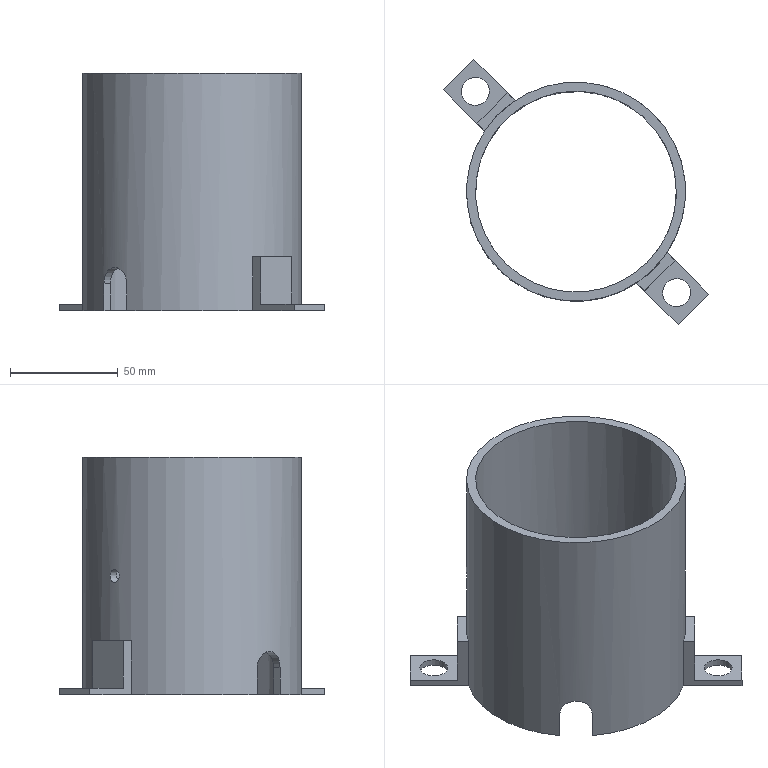Part | NX | features solid 2 | 1 solid | 26 faces | box 123.037 x 123.037 x 110 mm | volume 145297 mm3 | plane 19 | cylinder 7 | commonest cylinder face diameters 13 x2 15 x2 6 x1 93.2 x1 101.6 x1
STEP:
#1=CARTESIAN_POINT('',(-1217.073,-302.927,-100.));
#2=VERTEX_POINT('',#1);
#3=CARTESIAN_POINT('',(-1221.669,-298.331,-100.));
#4=DIRECTION('',(0.,0.,1.));
#5=DIRECTION('',(0.7071,-0.7071,0.));
#6=AXIS2_PLACEMENT_3D('',#3,#4,#5);
#7=CIRCLE('',#6,6.5);
#8=EDGE_CURVE('',#2,#2,#7,.T.);
#9=ORIENTED_EDGE('',*,*,#8,.T.);
#10=EDGE_LOOP('',(#9));
#11=FACE_BOUND('',#10,.T.);
#12=CARTESIAN_POINT('',(-1144.776,-304.169,-100.));
#13=VERTEX_POINT('',#12);
#14=CARTESIAN_POINT('',(-1203.147,-302.711,-100.));
#15=VERTEX_POINT('',#14);
#16=CARTESIAN_POINT('',(-1175.,-345.,-100.));
#17=DIRECTION('',(0.,0.,1.));
#18=DIRECTION('',(0.7071,-0.7071,0.));
#19=AXIS2_PLACEMENT_3D('',#16,#17,#18);
#20=CIRCLE('',#19,50.8);
#21=EDGE_CURVE('',#13,#15,#20,.T.);
#22=ORIENTED_EDGE('',*,*,#21,.F.);
#23=CARTESIAN_POINT('',(-1147.782,-307.175,-100.));
#24=VERTEX_POINT('',#23);
#25=CARTESIAN_POINT('',(-1180.303,-339.697,-100.));
#26=DIRECTION('',(-0.7071,-0.7071,0.));
#27=VECTOR('',#26,1000.);
#28=LINE('',#25,#27);
#29=EDGE_CURVE('',#13,#24,#28,.T.);
#30=ORIENTED_EDGE('',*,*,#29,.T.);
#31=CARTESIAN_POINT('',(-1212.825,-372.218,-100.));
#32=VERTEX_POINT('',#31);
#33=CARTESIAN_POINT('',(-1175.,-345.,-100.));
#34=DIRECTION('',(0.,0.,1.));
#35=DIRECTION('',(0.7071,-0.7071,0.));
#36=AXIS2_PLACEMENT_3D('',#33,#34,#35);
#37=CIRCLE('',#36,46.6);
#38=EDGE_CURVE('',#24,#32,#37,.T.);
#39=ORIENTED_EDGE('',*,*,#38,.T.);
#40=CARTESIAN_POINT('',(-1215.831,-375.224,-100.));
#41=VERTEX_POINT('',#40);
#42=CARTESIAN_POINT('',(-1180.303,-339.697,-100.));
#43=DIRECTION('',(-0.7071,-0.7071,0.));
#44=VECTOR('',#43,1000.);
#45=LINE('',#42,#44);
#46=EDGE_CURVE('',#32,#41,#45,.T.);
#47=ORIENTED_EDGE('',*,*,#46,.T.);
#48=CARTESIAN_POINT('',(-1217.289,-316.853,-100.));
#49=VERTEX_POINT('',#48);
#50=CARTESIAN_POINT('',(-1175.,-345.,-100.));
#51=DIRECTION('',(0.,0.,1.));
#52=DIRECTION('',(0.7071,-0.7071,0.));
#53=AXIS2_PLACEMENT_3D('',#50,#51,#52);
#54=CIRCLE('',#53,50.8);
#55=EDGE_CURVE('',#49,#41,#54,.T.);
#56=ORIENTED_EDGE('',*,*,#55,.F.);
#57=CARTESIAN_POINT('',(-1236.518,-297.624,-100.));
#58=VERTEX_POINT('',#57);
#59=CARTESIAN_POINT('',(-1226.619,-307.523,-100.));
#60=DIRECTION('',(0.7071,-0.7071,0.));
#61=VECTOR('',#60,1000.);
#62=LINE('',#59,#61);
#63=EDGE_CURVE('',#58,#49,#62,.T.);
#64=ORIENTED_EDGE('',*,*,#63,.F.);
#65=CARTESIAN_POINT('',(-1222.376,-283.482,-100.));
#66=VERTEX_POINT('',#65);
#67=CARTESIAN_POINT('',(-1236.518,-297.624,-100.));
#68=DIRECTION('',(0.7071,0.7071,0.));
#69=VECTOR('',#68,1000.);
#70=LINE('',#67,#69);
#71=EDGE_CURVE('',#58,#66,#70,.T.);
#72=ORIENTED_EDGE('',*,*,#71,.T.);
#73=CARTESIAN_POINT('',(-1206.113,-299.745,-100.));
#74=DIRECTION('',(-0.7071,0.7071,0.));
#75=VECTOR('',#74,1000.);
#76=LINE('',#73,#75);
#77=EDGE_CURVE('',#15,#66,#76,.T.);
#78=ORIENTED_EDGE('',*,*,#77,.F.);
#79=EDGE_LOOP('',(#22,#30,#39,#47,#56,#64,#72,#78));
#80=FACE_BOUND('',#79,.T.);
#81=CARTESIAN_POINT('',(-1175.,-345.,-100.));
#82=DIRECTION('',(0.,0.,1.));
#83=DIRECTION('',(0.7071,-0.7071,0.));
#84=AXIS2_PLACEMENT_3D('',#81,#82,#83);
#85=PLANE('',#84);
#86=ADVANCED_FACE('',(#11,#80),#85,.F.);
#87=CARTESIAN_POINT('',(-1211.112,-309.271,-47.988));
#88=VERTEX_POINT('',#87);
#89=CARTESIAN_POINT('',(-1212.688,-310.926,-47.127));
#90=CARTESIAN_POINT('',(-1211.147,-309.276,-48.312));
#91=CARTESIAN_POINT('',(-1209.392,-307.596,-47.552));
#92=CARTESIAN_POINT('',(-1208.503,-306.816,-45.302));
#93=CARTESIAN_POINT('',(-1209.075,-307.313,-42.871));
#94=CARTESIAN_POINT('',(-1210.724,-308.852,-41.689));
#95=CARTESIAN_POINT('',(-1212.402,-310.605,-42.445));
#96=CARTESIAN_POINT('',(-1213.185,-311.498,-44.697));
#97=CARTESIAN_POINT('',(-1212.688,-310.926,-47.127));
#98=CARTESIAN_POINT('',(-1211.147,-309.276,-48.312));
#99=CARTESIAN_POINT('',(-1209.392,-307.596,-47.552));
#100=B_SPLINE_CURVE_WITH_KNOTS('',3,(#89,#90,#91,#92,#93,#94,#95,#96,#97,#98,#99),.UNSPECIFIED.,.T.,.F.,(1,1,1,1,1,1,1,1,1,1,1,1,1,1,1),(-0.007035,-0.00469,-0.002345,0.,0.002345,0.00469,0.007035,0.00938,0.01173,0.01407,0.01642,0.01876,0.02111,0.02345,0.0258),.UNSPECIFIED.);
#101=EDGE_CURVE('',#88,#88,#100,.T.);
#102=ORIENTED_EDGE('',*,*,#101,.T.);
#103=EDGE_LOOP('',(#102));
#104=FACE_BOUND('',#103,.T.);
#105=CARTESIAN_POINT('',(-1139.079,-380.921,10.));
#106=VERTEX_POINT('',#105);
#107=CARTESIAN_POINT('',(-1175.,-345.,10.));
#108=DIRECTION('',(0.,0.,1.));
#109=DIRECTION('',(0.7071,-0.7071,0.));
#110=AXIS2_PLACEMENT_3D('',#107,#108,#109);
#111=CIRCLE('',#110,50.8);
#112=EDGE_CURVE('',#106,#106,#111,.T.);
#113=ORIENTED_EDGE('',*,*,#112,.F.);
#114=EDGE_LOOP('',(#113));
#115=FACE_BOUND('',#114,.T.);
#116=CARTESIAN_POINT('',(-1134.169,-314.776,-87.5));
#117=VERTEX_POINT('',#116);
#118=CARTESIAN_POINT('',(-1144.776,-304.169,-87.5));
#119=VERTEX_POINT('',#118);
#120=CARTESIAN_POINT('',(-1134.169,-314.776,-87.5));
#121=CARTESIAN_POINT('',(-1134.169,-314.776,-85.515));
#122=CARTESIAN_POINT('',(-1135.121,-313.429,-81.635));
#123=CARTESIAN_POINT('',(-1138.975,-308.987,-79.184));
#124=CARTESIAN_POINT('',(-1143.428,-305.121,-81.63));
#125=CARTESIAN_POINT('',(-1144.776,-304.169,-85.515));
#126=CARTESIAN_POINT('',(-1144.776,-304.169,-87.5));
#127=B_SPLINE_CURVE_WITH_KNOTS('',3,(#120,#121,#122,#123,#124,#125,#126),.UNSPECIFIED.,.F.,.F.,(4,1,1,1,4),(0.,0.005869,0.01174,0.01761,0.02347),.UNSPECIFIED.);
#128=EDGE_CURVE('',#117,#119,#127,.T.);
#129=ORIENTED_EDGE('',*,*,#128,.T.);
#130=CARTESIAN_POINT('',(-1144.776,-304.169,-93.75));
#131=DIRECTION('',(0.,0.,-1.));
#132=VECTOR('',#131,1000.);
#133=LINE('',#130,#132);
#134=EDGE_CURVE('',#119,#13,#133,.T.);
#135=ORIENTED_EDGE('',*,*,#134,.T.);
#136=ORIENTED_EDGE('',*,*,#21,.T.);
#137=CARTESIAN_POINT('',(-1203.147,-302.711,-75.));
#138=VERTEX_POINT('',#137);
#139=CARTESIAN_POINT('',(-1203.147,-302.711,-87.5));
#140=DIRECTION('',(0.,0.,-1.));
#141=VECTOR('',#140,1000.);
#142=LINE('',#139,#141);
#143=EDGE_CURVE('',#138,#15,#142,.T.);
#144=ORIENTED_EDGE('',*,*,#143,.F.);
#145=CARTESIAN_POINT('',(-1217.289,-316.853,-75.));
#146=VERTEX_POINT('',#145);
#147=CARTESIAN_POINT('',(-1175.,-345.,-75.));
#148=DIRECTION('',(0.,0.,1.));
#149=DIRECTION('',(0.7071,-0.7071,0.));
#150=AXIS2_PLACEMENT_3D('',#147,#148,#149);
#151=CIRCLE('',#150,50.8);
#152=EDGE_CURVE('',#138,#146,#151,.T.);
#153=ORIENTED_EDGE('',*,*,#152,.T.);
#154=CARTESIAN_POINT('',(-1217.289,-316.853,-87.5));
#155=DIRECTION('',(0.,0.,-1.));
#156=VECTOR('',#155,1000.);
#157=LINE('',#154,#156);
#158=EDGE_CURVE('',#49,#146,#157,.F.);
#159=ORIENTED_EDGE('',*,*,#158,.F.);
#160=ORIENTED_EDGE('',*,*,#55,.T.);
#161=CARTESIAN_POINT('',(-1215.831,-375.224,-87.5));
#162=VERTEX_POINT('',#161);
#163=CARTESIAN_POINT('',(-1215.831,-375.224,-93.75));
#164=DIRECTION('',(0.,0.,-1.));
#165=VECTOR('',#164,1000.);
#166=LINE('',#163,#165);
#167=EDGE_CURVE('',#41,#162,#166,.F.);
#168=ORIENTED_EDGE('',*,*,#167,.T.);
#169=CARTESIAN_POINT('',(-1205.224,-385.831,-87.5));
#170=VERTEX_POINT('',#169);
#171=CARTESIAN_POINT('',(-1215.831,-375.224,-87.5));
#172=CARTESIAN_POINT('',(-1215.831,-375.224,-85.515));
#173=CARTESIAN_POINT('',(-1214.879,-376.571,-81.635));
#174=CARTESIAN_POINT('',(-1211.025,-381.013,-79.184));
#175=CARTESIAN_POINT('',(-1206.572,-384.879,-81.63));
#176=CARTESIAN_POINT('',(-1205.224,-385.831,-85.515));
#177=CARTESIAN_POINT('',(-1205.224,-385.831,-87.5));
#178=B_SPLINE_CURVE_WITH_KNOTS('',3,(#171,#172,#173,#174,#175,#176,#177),.UNSPECIFIED.,.F.,.F.,(4,1,1,1,4),(0.,0.005869,0.01174,0.01761,0.02347),.UNSPECIFIED.);
#179=EDGE_CURVE('',#162,#170,#178,.T.);
#180=ORIENTED_EDGE('',*,*,#179,.T.);
#181=CARTESIAN_POINT('',(-1205.224,-385.831,-100.));
#182=VERTEX_POINT('',#181);
#183=CARTESIAN_POINT('',(-1205.224,-385.831,-93.75));
#184=DIRECTION('',(0.,0.,-1.));
#185=VECTOR('',#184,1000.);
#186=LINE('',#183,#185);
#187=EDGE_CURVE('',#170,#182,#186,.T.);
#188=ORIENTED_EDGE('',*,*,#187,.T.);
#189=CARTESIAN_POINT('',(-1146.853,-387.289,-100.));
#190=VERTEX_POINT('',#189);
#191=CARTESIAN_POINT('',(-1175.,-345.,-100.));
#192=DIRECTION('',(0.,0.,1.));
#193=DIRECTION('',(0.7071,-0.7071,0.));
#194=AXIS2_PLACEMENT_3D('',#191,#192,#193);
#195=CIRCLE('',#194,50.8);
#196=EDGE_CURVE('',#182,#190,#195,.T.);
#197=ORIENTED_EDGE('',*,*,#196,.T.);
#198=CARTESIAN_POINT('',(-1146.853,-387.289,-75.));
#199=VERTEX_POINT('',#198);
#200=CARTESIAN_POINT('',(-1146.853,-387.289,-87.5));
#201=DIRECTION('',(0.,0.,-1.));
#202=VECTOR('',#201,1000.);
#203=LINE('',#200,#202);
#204=EDGE_CURVE('',#199,#190,#203,.T.);
#205=ORIENTED_EDGE('',*,*,#204,.F.);
#206=CARTESIAN_POINT('',(-1132.711,-373.147,-75.));
#207=VERTEX_POINT('',#206);
#208=CARTESIAN_POINT('',(-1175.,-345.,-75.));
#209=DIRECTION('',(0.,0.,1.));
#210=DIRECTION('',(0.7071,-0.7071,0.));
#211=AXIS2_PLACEMENT_3D('',#208,#209,#210);
#212=CIRCLE('',#211,50.8);
#213=EDGE_CURVE('',#199,#207,#212,.T.);
#214=ORIENTED_EDGE('',*,*,#213,.T.);
#215=CARTESIAN_POINT('',(-1132.711,-373.147,-100.));
#216=VERTEX_POINT('',#215);
#217=CARTESIAN_POINT('',(-1132.711,-373.147,-87.5));
#218=DIRECTION('',(0.,0.,-1.));
#219=VECTOR('',#218,1000.);
#220=LINE('',#217,#219);
#221=EDGE_CURVE('',#216,#207,#220,.F.);
#222=ORIENTED_EDGE('',*,*,#221,.F.);
#223=CARTESIAN_POINT('',(-1134.169,-314.776,-100.));
#224=VERTEX_POINT('',#223);
#225=CARTESIAN_POINT('',(-1175.,-345.,-100.));
#226=DIRECTION('',(0.,0.,1.));
#227=DIRECTION('',(0.7071,-0.7071,0.));
#228=AXIS2_PLACEMENT_3D('',#225,#226,#227);
#229=CIRCLE('',#228,50.8);
#230=EDGE_CURVE('',#216,#224,#229,.T.);
#231=ORIENTED_EDGE('',*,*,#230,.T.);
#232=CARTESIAN_POINT('',(-1134.169,-314.776,-93.75));
#233=DIRECTION('',(0.,0.,-1.));
#234=VECTOR('',#233,1000.);
#235=LINE('',#232,#234);
#236=EDGE_CURVE('',#224,#117,#235,.F.);
#237=ORIENTED_EDGE('',*,*,#236,.T.);
#238=EDGE_LOOP('',(#129,#135,#136,#144,#153,#159,#160,#168,#180,#188,#197,#205,#214,#222,#231,#237));
#239=FACE_BOUND('',#238,.T.);
#240=CARTESIAN_POINT('',(-1175.,-345.,10.));
#241=DIRECTION('',(0.,0.,-1.));
#242=DIRECTION('',(-0.7071,0.7071,0.));
#243=AXIS2_PLACEMENT_3D('',#240,#241,#242);
#244=CYLINDRICAL_SURFACE('',#243,50.8);
#245=ADVANCED_FACE('',(#104,#115,#239),#244,.T.);
#246=CARTESIAN_POINT('',(-1147.782,-307.175,-87.5));
#247=VERTEX_POINT('',#246);
#248=CARTESIAN_POINT('',(-1147.782,-307.175,-93.75));
#249=DIRECTION('',(0.,0.,-1.));
#250=VECTOR('',#249,1000.);
#251=LINE('',#248,#250);
#252=EDGE_CURVE('',#247,#24,#251,.T.);
#253=ORIENTED_EDGE('',*,*,#252,.F.);
#254=CARTESIAN_POINT('',(-1137.175,-317.782,-87.5));
#255=VERTEX_POINT('',#254);
#256=CARTESIAN_POINT('',(-1137.175,-317.782,-87.5));
#257=CARTESIAN_POINT('',(-1137.175,-317.782,-85.515));
#258=CARTESIAN_POINT('',(-1138.108,-316.416,-81.635));
#259=CARTESIAN_POINT('',(-1141.936,-311.948,-79.184));
#260=CARTESIAN_POINT('',(-1146.415,-308.108,-81.63));
#261=CARTESIAN_POINT('',(-1147.782,-307.175,-85.515));
#262=CARTESIAN_POINT('',(-1147.782,-307.175,-87.5));
#263=B_SPLINE_CURVE_WITH_KNOTS('',3,(#256,#257,#258,#259,#260,#261,#262),.UNSPECIFIED.,.F.,.F.,(4,1,1,1,4),(0.,0.00587,0.01174,0.01761,0.02348),.UNSPECIFIED.);
#264=EDGE_CURVE('',#255,#247,#263,.T.);
#265=ORIENTED_EDGE('',*,*,#264,.F.);
#266=CARTESIAN_POINT('',(-1137.175,-317.782,-100.));
#267=VERTEX_POINT('',#266);
#268=CARTESIAN_POINT('',(-1137.175,-317.782,-93.75));
#269=DIRECTION('',(0.,0.,-1.));
#270=VECTOR('',#269,1000.);
#271=LINE('',#268,#270);
#272=EDGE_CURVE('',#267,#255,#271,.F.);
#273=ORIENTED_EDGE('',*,*,#272,.F.);
#274=CARTESIAN_POINT('',(-1202.218,-382.825,-100.));
#275=VERTEX_POINT('',#274);
#276=CARTESIAN_POINT('',(-1175.,-345.,-100.));
#277=DIRECTION('',(0.,0.,1.));
#278=DIRECTION('',(0.7071,-0.7071,0.));
#279=AXIS2_PLACEMENT_3D('',#276,#277,#278);
#280=CIRCLE('',#279,46.6);
#281=EDGE_CURVE('',#275,#267,#280,.T.);
#282=ORIENTED_EDGE('',*,*,#281,.F.);
#283=CARTESIAN_POINT('',(-1202.218,-382.825,-87.5));
#284=VERTEX_POINT('',#283);
#285=CARTESIAN_POINT('',(-1202.218,-382.825,-93.75));
#286=DIRECTION('',(0.,0.,-1.));
#287=VECTOR('',#286,1000.);
#288=LINE('',#285,#287);
#289=EDGE_CURVE('',#284,#275,#288,.T.);
#290=ORIENTED_EDGE('',*,*,#289,.F.);
#291=CARTESIAN_POINT('',(-1212.825,-372.218,-87.5));
#292=VERTEX_POINT('',#291);
#293=CARTESIAN_POINT('',(-1212.825,-372.218,-87.5));
#294=CARTESIAN_POINT('',(-1212.825,-372.218,-85.515));
#295=CARTESIAN_POINT('',(-1211.892,-373.584,-81.635));
#296=CARTESIAN_POINT('',(-1208.064,-378.052,-79.184));
#297=CARTESIAN_POINT('',(-1203.585,-381.892,-81.63));
#298=CARTESIAN_POINT('',(-1202.218,-382.825,-85.515));
#299=CARTESIAN_POINT('',(-1202.218,-382.825,-87.5));
#300=B_SPLINE_CURVE_WITH_KNOTS('',3,(#293,#294,#295,#296,#297,#298,#299),.UNSPECIFIED.,.F.,.F.,(4,1,1,1,4),(0.,0.00587,0.01174,0.01761,0.02348),.UNSPECIFIED.);
#301=EDGE_CURVE('',#292,#284,#300,.T.);
#302=ORIENTED_EDGE('',*,*,#301,.F.);
#303=CARTESIAN_POINT('',(-1212.825,-372.218,-93.75));
#304=DIRECTION('',(0.,0.,-1.));
#305=VECTOR('',#304,1000.);
#306=LINE('',#303,#305);
#307=EDGE_CURVE('',#32,#292,#306,.F.);
#308=ORIENTED_EDGE('',*,*,#307,.F.);
#309=ORIENTED_EDGE('',*,*,#38,.F.);
#310=EDGE_LOOP('',(#253,#265,#273,#282,#290,#302,#308,#309));
#311=FACE_BOUND('',#310,.T.);
#312=CARTESIAN_POINT('',(-1208.146,-312.245,-47.987));
#313=VERTEX_POINT('',#312);
#314=CARTESIAN_POINT('',(-1209.717,-313.902,-47.122));
#315=CARTESIAN_POINT('',(-1208.184,-312.249,-48.311));
#316=CARTESIAN_POINT('',(-1206.424,-310.571,-47.556));
#317=CARTESIAN_POINT('',(-1205.526,-309.793,-45.309));
#318=CARTESIAN_POINT('',(-1206.098,-310.283,-42.876));
#319=CARTESIAN_POINT('',(-1207.751,-311.816,-41.69));
#320=CARTESIAN_POINT('',(-1209.427,-313.574,-42.441));
#321=CARTESIAN_POINT('',(-1210.207,-314.474,-44.69));
#322=CARTESIAN_POINT('',(-1209.717,-313.902,-47.122));
#323=CARTESIAN_POINT('',(-1208.184,-312.249,-48.311));
#324=CARTESIAN_POINT('',(-1206.424,-310.571,-47.556));
#325=B_SPLINE_CURVE_WITH_KNOTS('',3,(#314,#315,#316,#317,#318,#319,#320,#321,#322,#323,#324),.UNSPECIFIED.,.T.,.F.,(1,1,1,1,1,1,1,1,1,1,1,1,1,1,1),(-0.007036,-0.00469,-0.002345,0.,0.002345,0.00469,0.007036,0.009381,0.01173,0.01407,0.01642,0.01876,0.02111,0.02345,0.0258),.UNSPECIFIED.);
#326=EDGE_CURVE('',#313,#313,#325,.T.);
#327=ORIENTED_EDGE('',*,*,#326,.F.);
#328=EDGE_LOOP('',(#327));
#329=FACE_BOUND('',#328,.T.);
#330=CARTESIAN_POINT('',(-1142.049,-377.951,10.));
#331=VERTEX_POINT('',#330);
#332=CARTESIAN_POINT('',(-1175.,-345.,10.));
#333=DIRECTION('',(0.,0.,1.));
#334=DIRECTION('',(0.7071,-0.7071,0.));
#335=AXIS2_PLACEMENT_3D('',#332,#333,#334);
#336=CIRCLE('',#335,46.6);
#337=EDGE_CURVE('',#331,#331,#336,.T.);
#338=ORIENTED_EDGE('',*,*,#337,.T.);
#339=EDGE_LOOP('',(#338));
#340=FACE_BOUND('',#339,.T.);
#341=CARTESIAN_POINT('',(-1175.,-345.,10.));
#342=DIRECTION('',(0.,0.,-1.));
#343=DIRECTION('',(-0.7071,0.7071,0.));
#344=AXIS2_PLACEMENT_3D('',#341,#342,#343);
#345=CYLINDRICAL_SURFACE('',#344,46.6);
#346=ADVANCED_FACE('',(#311,#329,#340),#345,.F.);
#347=ORIENTED_EDGE('',*,*,#337,.F.);
#348=EDGE_LOOP('',(#347));
#349=FACE_BOUND('',#348,.T.);
#350=ORIENTED_EDGE('',*,*,#112,.T.);
#351=EDGE_LOOP('',(#350));
#352=FACE_BOUND('',#351,.T.);
#353=CARTESIAN_POINT('',(-1175.,-345.,10.));
#354=DIRECTION('',(0.,0.,1.));
#355=DIRECTION('',(0.7071,-0.7071,0.));
#356=AXIS2_PLACEMENT_3D('',#353,#354,#355);
#357=PLANE('',#356);
#358=ADVANCED_FACE('',(#349,#352),#357,.T.);
#359=ORIENTED_EDGE('',*,*,#281,.T.);
#360=CARTESIAN_POINT('',(-1169.697,-350.303,-100.));
#361=DIRECTION('',(0.7071,0.7071,0.));
#362=VECTOR('',#361,1000.);
#363=LINE('',#360,#362);
#364=EDGE_CURVE('',#267,#224,#363,.T.);
#365=ORIENTED_EDGE('',*,*,#364,.T.);
#366=ORIENTED_EDGE('',*,*,#230,.F.);
#367=CARTESIAN_POINT('',(-1113.482,-392.376,-100.));
#368=VERTEX_POINT('',#367);
#369=CARTESIAN_POINT('',(-1123.381,-382.477,-100.));
#370=DIRECTION('',(-0.7071,0.7071,0.));
#371=VECTOR('',#370,1000.);
#372=LINE('',#369,#371);
#373=EDGE_CURVE('',#368,#216,#372,.T.);
#374=ORIENTED_EDGE('',*,*,#373,.F.);
#375=CARTESIAN_POINT('',(-1127.624,-406.518,-100.));
#376=VERTEX_POINT('',#375);
#377=CARTESIAN_POINT('',(-1113.482,-392.376,-100.));
#378=DIRECTION('',(-0.7071,-0.7071,0.));
#379=VECTOR('',#378,1000.);
#380=LINE('',#377,#379);
#381=EDGE_CURVE('',#368,#376,#380,.T.);
#382=ORIENTED_EDGE('',*,*,#381,.T.);
#383=CARTESIAN_POINT('',(-1143.887,-390.255,-100.));
#384=DIRECTION('',(0.7071,-0.7071,0.));
#385=VECTOR('',#384,1000.);
#386=LINE('',#383,#385);
#387=EDGE_CURVE('',#190,#376,#386,.T.);
#388=ORIENTED_EDGE('',*,*,#387,.F.);
#389=ORIENTED_EDGE('',*,*,#196,.F.);
#390=CARTESIAN_POINT('',(-1169.697,-350.303,-100.));
#391=DIRECTION('',(0.7071,0.7071,0.));
#392=VECTOR('',#391,1000.);
#393=LINE('',#390,#392);
#394=EDGE_CURVE('',#182,#275,#393,.T.);
#395=ORIENTED_EDGE('',*,*,#394,.T.);
#396=EDGE_LOOP('',(#359,#365,#366,#374,#382,#388,#389,#395));
#397=FACE_BOUND('',#396,.T.);
#398=CARTESIAN_POINT('',(-1123.735,-396.265,-100.));
#399=VERTEX_POINT('',#398);
#400=CARTESIAN_POINT('',(-1128.331,-391.669,-100.));
#401=DIRECTION('',(0.,0.,1.));
#402=DIRECTION('',(0.7071,-0.7071,0.));
#403=AXIS2_PLACEMENT_3D('',#400,#401,#402);
#404=CIRCLE('',#403,6.5);
#405=EDGE_CURVE('',#399,#399,#404,.T.);
#406=ORIENTED_EDGE('',*,*,#405,.T.);
#407=EDGE_LOOP('',(#406));
#408=FACE_BOUND('',#407,.T.);
#409=CARTESIAN_POINT('',(-1175.,-345.,-100.));
#410=DIRECTION('',(0.,0.,1.));
#411=DIRECTION('',(0.7071,-0.7071,0.));
#412=AXIS2_PLACEMENT_3D('',#409,#410,#411);
#413=PLANE('',#412);
#414=ADVANCED_FACE('',(#397,#408),#413,.F.);
#415=CARTESIAN_POINT('',(-1206.82,-299.038,-75.));
#416=VERTEX_POINT('',#415);
#417=CARTESIAN_POINT('',(-1220.962,-313.18,-75.));
#418=VERTEX_POINT('',#417);
#419=CARTESIAN_POINT('',(-1206.82,-299.038,-75.));
#420=DIRECTION('',(-0.7071,-0.7071,0.));
#421=VECTOR('',#420,1000.);
#422=LINE('',#419,#421);
#423=EDGE_CURVE('',#416,#418,#422,.T.);
#424=ORIENTED_EDGE('',*,*,#423,.T.);
#425=CARTESIAN_POINT('',(-1226.619,-307.523,-75.));
#426=DIRECTION('',(0.7071,-0.7071,0.));
#427=VECTOR('',#426,1000.);
#428=LINE('',#425,#427);
#429=EDGE_CURVE('',#418,#146,#428,.T.);
#430=ORIENTED_EDGE('',*,*,#429,.T.);
#431=ORIENTED_EDGE('',*,*,#152,.F.);
#432=CARTESIAN_POINT('',(-1206.113,-299.745,-75.));
#433=DIRECTION('',(-0.7071,0.7071,0.));
#434=VECTOR('',#433,1000.);
#435=LINE('',#432,#434);
#436=EDGE_CURVE('',#138,#416,#435,.T.);
#437=ORIENTED_EDGE('',*,*,#436,.T.);
#438=EDGE_LOOP('',(#424,#430,#431,#437));
#439=FACE_BOUND('',#438,.T.);
#440=CARTESIAN_POINT('',(-1226.619,-307.523,-75.));
#441=DIRECTION('',(0.,0.,1.));
#442=DIRECTION('',(0.7071,-0.7071,0.));
#443=AXIS2_PLACEMENT_3D('',#440,#441,#442);
#444=PLANE('',#443);
#445=ADVANCED_FACE('',(#439),#444,.T.);
#446=ORIENTED_EDGE('',*,*,#63,.T.);
#447=ORIENTED_EDGE('',*,*,#158,.T.);
#448=ORIENTED_EDGE('',*,*,#429,.F.);
#449=CARTESIAN_POINT('',(-1220.962,-313.18,-97.));
#450=VERTEX_POINT('',#449);
#451=CARTESIAN_POINT('',(-1220.962,-313.18,-75.));
#452=DIRECTION('',(0.,0.,-1.));
#453=VECTOR('',#452,1000.);
#454=LINE('',#451,#453);
#455=EDGE_CURVE('',#418,#450,#454,.T.);
#456=ORIENTED_EDGE('',*,*,#455,.T.);
#457=CARTESIAN_POINT('',(-1236.518,-297.624,-97.));
#458=VERTEX_POINT('',#457);
#459=CARTESIAN_POINT('',(-1226.619,-307.523,-97.));
#460=DIRECTION('',(-0.7071,0.7071,0.));
#461=VECTOR('',#460,1000.);
#462=LINE('',#459,#461);
#463=EDGE_CURVE('',#450,#458,#462,.T.);
#464=ORIENTED_EDGE('',*,*,#463,.T.);
#465=CARTESIAN_POINT('',(-1236.518,-297.624,-97.));
#466=DIRECTION('',(0.,0.,-1.));
#467=VECTOR('',#466,1000.);
#468=LINE('',#465,#467);
#469=EDGE_CURVE('',#458,#58,#468,.T.);
#470=ORIENTED_EDGE('',*,*,#469,.T.);
#471=EDGE_LOOP('',(#446,#447,#448,#456,#464,#470));
#472=FACE_BOUND('',#471,.T.);
#473=CARTESIAN_POINT('',(-1226.619,-307.523,-75.));
#474=DIRECTION('',(0.7071,0.7071,0.));
#475=DIRECTION('',(-0.7071,0.7071,0.));
#476=AXIS2_PLACEMENT_3D('',#473,#474,#475);
#477=PLANE('',#476);
#478=ADVANCED_FACE('',(#472),#477,.F.);
#479=ORIENTED_EDGE('',*,*,#436,.F.);
#480=ORIENTED_EDGE('',*,*,#143,.T.);
#481=ORIENTED_EDGE('',*,*,#77,.T.);
#482=CARTESIAN_POINT('',(-1222.376,-283.482,-97.));
#483=VERTEX_POINT('',#482);
#484=CARTESIAN_POINT('',(-1222.376,-283.482,-97.));
#485=DIRECTION('',(0.,0.,-1.));
#486=VECTOR('',#485,1000.);
#487=LINE('',#484,#486);
#488=EDGE_CURVE('',#483,#66,#487,.T.);
#489=ORIENTED_EDGE('',*,*,#488,.F.);
#490=CARTESIAN_POINT('',(-1206.82,-299.038,-97.));
#491=VERTEX_POINT('',#490);
#492=CARTESIAN_POINT('',(-1228.033,-277.825,-97.));
#493=DIRECTION('',(0.7071,-0.7071,0.));
#494=VECTOR('',#493,1000.);
#495=LINE('',#492,#494);
#496=EDGE_CURVE('',#483,#491,#495,.T.);
#497=ORIENTED_EDGE('',*,*,#496,.T.);
#498=CARTESIAN_POINT('',(-1206.82,-299.038,-75.));
#499=DIRECTION('',(0.,0.,-1.));
#500=VECTOR('',#499,1000.);
#501=LINE('',#498,#500);
#502=EDGE_CURVE('',#416,#491,#501,.T.);
#503=ORIENTED_EDGE('',*,*,#502,.F.);
#504=EDGE_LOOP('',(#479,#480,#481,#489,#497,#503));
#505=FACE_BOUND('',#504,.T.);
#506=CARTESIAN_POINT('',(-1206.113,-299.745,-75.));
#507=DIRECTION('',(-0.7071,-0.7071,0.));
#508=DIRECTION('',(0.7071,-0.7071,0.));
#509=AXIS2_PLACEMENT_3D('',#506,#507,#508);
#510=PLANE('',#509);
#511=ADVANCED_FACE('',(#505),#510,.F.);
#512=ORIENTED_EDGE('',*,*,#502,.T.);
#513=CARTESIAN_POINT('',(-1206.82,-299.038,-97.));
#514=DIRECTION('',(-0.7071,-0.7071,0.));
#515=VECTOR('',#514,1000.);
#516=LINE('',#513,#515);
#517=EDGE_CURVE('',#491,#450,#516,.T.);
#518=ORIENTED_EDGE('',*,*,#517,.T.);
#519=ORIENTED_EDGE('',*,*,#455,.F.);
#520=ORIENTED_EDGE('',*,*,#423,.F.);
#521=EDGE_LOOP('',(#512,#518,#519,#520));
#522=FACE_BOUND('',#521,.T.);
#523=CARTESIAN_POINT('',(-1206.82,-299.038,-75.));
#524=DIRECTION('',(0.7071,-0.7071,0.));
#525=DIRECTION('',(0.,0.,-1.));
#526=AXIS2_PLACEMENT_3D('',#523,#524,#525);
#527=PLANE('',#526);
#528=ADVANCED_FACE('',(#522),#527,.F.);
#529=CARTESIAN_POINT('',(-1143.18,-390.962,-75.));
#530=VERTEX_POINT('',#529);
#531=CARTESIAN_POINT('',(-1129.038,-376.82,-75.));
#532=VERTEX_POINT('',#531);
#533=CARTESIAN_POINT('',(-1143.18,-390.962,-75.));
#534=DIRECTION('',(0.7071,0.7071,0.));
#535=VECTOR('',#534,1000.);
#536=LINE('',#533,#535);
#537=EDGE_CURVE('',#530,#532,#536,.T.);
#538=ORIENTED_EDGE('',*,*,#537,.T.);
#539=CARTESIAN_POINT('',(-1123.381,-382.477,-75.));
#540=DIRECTION('',(-0.7071,0.7071,0.));
#541=VECTOR('',#540,1000.);
#542=LINE('',#539,#541);
#543=EDGE_CURVE('',#532,#207,#542,.T.);
#544=ORIENTED_EDGE('',*,*,#543,.T.);
#545=ORIENTED_EDGE('',*,*,#213,.F.);
#546=CARTESIAN_POINT('',(-1143.887,-390.255,-75.));
#547=DIRECTION('',(0.7071,-0.7071,0.));
#548=VECTOR('',#547,1000.);
#549=LINE('',#546,#548);
#550=EDGE_CURVE('',#199,#530,#549,.T.);
#551=ORIENTED_EDGE('',*,*,#550,.T.);
#552=EDGE_LOOP('',(#538,#544,#545,#551));
#553=FACE_BOUND('',#552,.T.);
#554=CARTESIAN_POINT('',(-1129.745,-376.113,-75.));
#555=DIRECTION('',(0.,0.,1.));
#556=DIRECTION('',(0.7071,-0.7071,0.));
#557=AXIS2_PLACEMENT_3D('',#554,#555,#556);
#558=PLANE('',#557);
#559=ADVANCED_FACE('',(#553),#558,.T.);
#560=ORIENTED_EDGE('',*,*,#373,.T.);
#561=ORIENTED_EDGE('',*,*,#221,.T.);
#562=ORIENTED_EDGE('',*,*,#543,.F.);
#563=CARTESIAN_POINT('',(-1129.038,-376.82,-97.));
#564=VERTEX_POINT('',#563);
#565=CARTESIAN_POINT('',(-1129.038,-376.82,-75.));
#566=DIRECTION('',(0.,0.,-1.));
#567=VECTOR('',#566,1000.);
#568=LINE('',#565,#567);
#569=EDGE_CURVE('',#532,#564,#568,.T.);
#570=ORIENTED_EDGE('',*,*,#569,.T.);
#571=CARTESIAN_POINT('',(-1113.482,-392.376,-97.));
#572=VERTEX_POINT('',#571);
#573=CARTESIAN_POINT('',(-1123.381,-382.477,-97.));
#574=DIRECTION('',(0.7071,-0.7071,0.));
#575=VECTOR('',#574,1000.);
#576=LINE('',#573,#575);
#577=EDGE_CURVE('',#564,#572,#576,.T.);
#578=ORIENTED_EDGE('',*,*,#577,.T.);
#579=CARTESIAN_POINT('',(-1113.482,-392.376,-97.));
#580=DIRECTION('',(0.,0.,-1.));
#581=VECTOR('',#580,1000.);
#582=LINE('',#579,#581);
#583=EDGE_CURVE('',#572,#368,#582,.T.);
#584=ORIENTED_EDGE('',*,*,#583,.T.);
#585=EDGE_LOOP('',(#560,#561,#562,#570,#578,#584));
#586=FACE_BOUND('',#585,.T.);
#587=CARTESIAN_POINT('',(-1123.381,-382.477,-75.));
#588=DIRECTION('',(-0.7071,-0.7071,0.));
#589=DIRECTION('',(0.7071,-0.7071,0.));
#590=AXIS2_PLACEMENT_3D('',#587,#588,#589);
#591=PLANE('',#590);
#592=ADVANCED_FACE('',(#586),#591,.F.);
#593=ORIENTED_EDGE('',*,*,#550,.F.);
#594=ORIENTED_EDGE('',*,*,#204,.T.);
#595=ORIENTED_EDGE('',*,*,#387,.T.);
#596=CARTESIAN_POINT('',(-1127.624,-406.518,-97.));
#597=VERTEX_POINT('',#596);
#598=CARTESIAN_POINT('',(-1127.624,-406.518,-97.));
#599=DIRECTION('',(0.,0.,-1.));
#600=VECTOR('',#599,1000.);
#601=LINE('',#598,#600);
#602=EDGE_CURVE('',#597,#376,#601,.T.);
#603=ORIENTED_EDGE('',*,*,#602,.F.);
#604=CARTESIAN_POINT('',(-1143.18,-390.962,-97.));
#605=VERTEX_POINT('',#604);
#606=CARTESIAN_POINT('',(-1121.967,-412.175,-97.));
#607=DIRECTION('',(-0.7071,0.7071,0.));
#608=VECTOR('',#607,1000.);
#609=LINE('',#606,#608);
#610=EDGE_CURVE('',#597,#605,#609,.T.);
#611=ORIENTED_EDGE('',*,*,#610,.T.);
#612=CARTESIAN_POINT('',(-1143.18,-390.962,-75.));
#613=DIRECTION('',(0.,0.,-1.));
#614=VECTOR('',#613,1000.);
#615=LINE('',#612,#614);
#616=EDGE_CURVE('',#530,#605,#615,.T.);
#617=ORIENTED_EDGE('',*,*,#616,.F.);
#618=EDGE_LOOP('',(#593,#594,#595,#603,#611,#617));
#619=FACE_BOUND('',#618,.T.);
#620=CARTESIAN_POINT('',(-1143.887,-390.255,-75.));
#621=DIRECTION('',(0.7071,0.7071,0.));
#622=DIRECTION('',(0.,0.,1.));
#623=AXIS2_PLACEMENT_3D('',#620,#621,#622);
#624=PLANE('',#623);
#625=ADVANCED_FACE('',(#619),#624,.F.);
#626=ORIENTED_EDGE('',*,*,#616,.T.);
#627=CARTESIAN_POINT('',(-1143.18,-390.962,-97.));
#628=DIRECTION('',(0.7071,0.7071,0.));
#629=VECTOR('',#628,1000.);
#630=LINE('',#627,#629);
#631=EDGE_CURVE('',#605,#564,#630,.T.);
#632=ORIENTED_EDGE('',*,*,#631,.T.);
#633=ORIENTED_EDGE('',*,*,#569,.F.);
#634=ORIENTED_EDGE('',*,*,#537,.F.);
#635=EDGE_LOOP('',(#626,#632,#633,#634));
#636=FACE_BOUND('',#635,.T.);
#637=CARTESIAN_POINT('',(-1143.18,-390.962,-75.));
#638=DIRECTION('',(-0.7071,0.7071,0.));
#639=DIRECTION('',(0.,0.,1.));
#640=AXIS2_PLACEMENT_3D('',#637,#638,#639);
#641=PLANE('',#640);
#642=ADVANCED_FACE('',(#636),#641,.F.);
#643=ORIENTED_EDGE('',*,*,#381,.F.);
#644=ORIENTED_EDGE('',*,*,#583,.F.);
#645=CARTESIAN_POINT('',(-1113.482,-392.376,-97.));
#646=DIRECTION('',(-0.7071,-0.7071,0.));
#647=VECTOR('',#646,1000.);
#648=LINE('',#645,#647);
#649=EDGE_CURVE('',#572,#597,#648,.T.);
#650=ORIENTED_EDGE('',*,*,#649,.T.);
#651=ORIENTED_EDGE('',*,*,#602,.T.);
#652=EDGE_LOOP('',(#643,#644,#650,#651));
#653=FACE_BOUND('',#652,.T.);
#654=CARTESIAN_POINT('',(-1113.482,-392.376,-97.));
#655=DIRECTION('',(0.7071,-0.7071,0.));
#656=DIRECTION('',(0.,0.,-1.));
#657=AXIS2_PLACEMENT_3D('',#654,#655,#656);
#658=PLANE('',#657);
#659=ADVANCED_FACE('',(#653),#658,.T.);
#660=CARTESIAN_POINT('',(-1123.735,-396.265,-97.));
#661=VERTEX_POINT('',#660);
#662=CARTESIAN_POINT('',(-1128.331,-391.669,-97.));
#663=DIRECTION('',(0.,0.,1.));
#664=DIRECTION('',(0.7071,-0.7071,0.));
#665=AXIS2_PLACEMENT_3D('',#662,#663,#664);
#666=CIRCLE('',#665,6.5);
#667=EDGE_CURVE('',#661,#661,#666,.T.);
#668=ORIENTED_EDGE('',*,*,#667,.T.);
#669=EDGE_LOOP('',(#668));
#670=FACE_BOUND('',#669,.T.);
#671=ORIENTED_EDGE('',*,*,#405,.F.);
#672=EDGE_LOOP('',(#671));
#673=FACE_BOUND('',#672,.T.);
#674=CARTESIAN_POINT('',(-1128.331,-391.669,-97.));
#675=DIRECTION('',(0.,0.,-1.));
#676=DIRECTION('',(-0.7071,0.7071,0.));
#677=AXIS2_PLACEMENT_3D('',#674,#675,#676);
#678=CYLINDRICAL_SURFACE('',#677,6.5);
#679=ADVANCED_FACE('',(#670,#673),#678,.F.);
#680=ORIENTED_EDGE('',*,*,#649,.F.);
#681=ORIENTED_EDGE('',*,*,#577,.F.);
#682=ORIENTED_EDGE('',*,*,#631,.F.);
#683=ORIENTED_EDGE('',*,*,#610,.F.);
#684=EDGE_LOOP('',(#680,#681,#682,#683));
#685=FACE_BOUND('',#684,.T.);
#686=ORIENTED_EDGE('',*,*,#667,.F.);
#687=EDGE_LOOP('',(#686));
#688=FACE_BOUND('',#687,.T.);
#689=CARTESIAN_POINT('',(-1121.967,-412.175,-97.));
#690=DIRECTION('',(0.,0.,-1.));
#691=DIRECTION('',(-0.7071,0.7071,0.));
#692=AXIS2_PLACEMENT_3D('',#689,#690,#691);
#693=PLANE('',#692);
#694=ADVANCED_FACE('',(#685,#688),#693,.F.);
#695=ORIENTED_EDGE('',*,*,#71,.F.);
#696=ORIENTED_EDGE('',*,*,#469,.F.);
#697=CARTESIAN_POINT('',(-1236.518,-297.624,-97.));
#698=DIRECTION('',(0.7071,0.7071,0.));
#699=VECTOR('',#698,1000.);
#700=LINE('',#697,#699);
#701=EDGE_CURVE('',#458,#483,#700,.T.);
#702=ORIENTED_EDGE('',*,*,#701,.T.);
#703=ORIENTED_EDGE('',*,*,#488,.T.);
#704=EDGE_LOOP('',(#695,#696,#702,#703));
#705=FACE_BOUND('',#704,.T.);
#706=CARTESIAN_POINT('',(-1236.518,-297.624,-97.));
#707=DIRECTION('',(-0.7071,0.7071,0.));
#708=DIRECTION('',(0.,0.,1.));
#709=AXIS2_PLACEMENT_3D('',#706,#707,#708);
#710=PLANE('',#709);
#711=ADVANCED_FACE('',(#705),#710,.T.);
#712=CARTESIAN_POINT('',(-1217.073,-302.927,-97.));
#713=VERTEX_POINT('',#712);
#714=CARTESIAN_POINT('',(-1221.669,-298.331,-97.));
#715=DIRECTION('',(0.,0.,1.));
#716=DIRECTION('',(0.7071,-0.7071,0.));
#717=AXIS2_PLACEMENT_3D('',#714,#715,#716);
#718=CIRCLE('',#717,6.5);
#719=EDGE_CURVE('',#713,#713,#718,.T.);
#720=ORIENTED_EDGE('',*,*,#719,.T.);
#721=EDGE_LOOP('',(#720));
#722=FACE_BOUND('',#721,.T.);
#723=ORIENTED_EDGE('',*,*,#8,.F.);
#724=EDGE_LOOP('',(#723));
#725=FACE_BOUND('',#724,.T.);
#726=CARTESIAN_POINT('',(-1221.669,-298.331,-97.));
#727=DIRECTION('',(0.,0.,-1.));
#728=DIRECTION('',(-0.7071,0.7071,0.));
#729=AXIS2_PLACEMENT_3D('',#726,#727,#728);
#730=CYLINDRICAL_SURFACE('',#729,6.5);
#731=ADVANCED_FACE('',(#722,#725),#730,.F.);
#732=ORIENTED_EDGE('',*,*,#701,.F.);
#733=ORIENTED_EDGE('',*,*,#463,.F.);
#734=ORIENTED_EDGE('',*,*,#517,.F.);
#735=ORIENTED_EDGE('',*,*,#496,.F.);
#736=EDGE_LOOP('',(#732,#733,#734,#735));
#737=FACE_BOUND('',#736,.T.);
#738=ORIENTED_EDGE('',*,*,#719,.F.);
#739=EDGE_LOOP('',(#738));
#740=FACE_BOUND('',#739,.T.);
#741=CARTESIAN_POINT('',(-1228.033,-277.825,-97.));
#742=DIRECTION('',(0.,0.,-1.));
#743=DIRECTION('',(-0.7071,0.7071,0.));
#744=AXIS2_PLACEMENT_3D('',#741,#742,#743);
#745=PLANE('',#744);
#746=ADVANCED_FACE('',(#737,#740),#745,.F.);
#747=ORIENTED_EDGE('',*,*,#326,.T.);
#748=EDGE_LOOP('',(#747));
#749=FACE_BOUND('',#748,.T.);
#750=ORIENTED_EDGE('',*,*,#101,.F.);
#751=EDGE_LOOP('',(#750));
#752=FACE_BOUND('',#751,.T.);
#753=CARTESIAN_POINT('',(-1175.,-345.,-45.));
#754=DIRECTION('',(-0.7071,0.7071,0.));
#755=DIRECTION('',(0.,0.,1.));
#756=AXIS2_PLACEMENT_3D('',#753,#754,#755);
#757=CYLINDRICAL_SURFACE('',#756,3.);
#758=ADVANCED_FACE('',(#749,#752),#757,.F.);
#759=CARTESIAN_POINT('',(-1180.303,-339.697,-87.5));
#760=DIRECTION('',(0.7071,0.7071,0.));
#761=VECTOR('',#760,1000.);
#762=LINE('',#759,#761);
#763=EDGE_CURVE('',#162,#292,#762,.T.);
#764=ORIENTED_EDGE('',*,*,#763,.T.);
#765=ORIENTED_EDGE('',*,*,#301,.T.);
#766=CARTESIAN_POINT('',(-1169.697,-350.303,-87.5));
#767=DIRECTION('',(0.7071,0.7071,0.));
#768=VECTOR('',#767,1000.);
#769=LINE('',#766,#768);
#770=EDGE_CURVE('',#170,#284,#769,.T.);
#771=ORIENTED_EDGE('',*,*,#770,.F.);
#772=ORIENTED_EDGE('',*,*,#179,.F.);
#773=EDGE_LOOP('',(#764,#765,#771,#772));
#774=FACE_BOUND('',#773,.T.);
#775=CARTESIAN_POINT('',(-1175.,-345.,-87.5));
#776=DIRECTION('',(0.7071,0.7071,0.));
#777=DIRECTION('',(0.,0.,1.));
#778=AXIS2_PLACEMENT_3D('',#775,#776,#777);
#779=CYLINDRICAL_SURFACE('',#778,7.5);
#780=ADVANCED_FACE('',(#774),#779,.F.);
#781=ORIENTED_EDGE('',*,*,#770,.T.);
#782=ORIENTED_EDGE('',*,*,#289,.T.);
#783=ORIENTED_EDGE('',*,*,#394,.F.);
#784=ORIENTED_EDGE('',*,*,#187,.F.);
#785=EDGE_LOOP('',(#781,#782,#783,#784));
#786=FACE_BOUND('',#785,.T.);
#787=CARTESIAN_POINT('',(-1169.697,-350.303,-100.));
#788=DIRECTION('',(0.7071,-0.7071,0.));
#789=DIRECTION('',(0.,0.,-1.));
#790=AXIS2_PLACEMENT_3D('',#787,#788,#789);
#791=PLANE('',#790);
#792=ADVANCED_FACE('',(#786),#791,.F.);
#793=ORIENTED_EDGE('',*,*,#46,.F.);
#794=ORIENTED_EDGE('',*,*,#307,.T.);
#795=ORIENTED_EDGE('',*,*,#763,.F.);
#796=ORIENTED_EDGE('',*,*,#167,.F.);
#797=EDGE_LOOP('',(#793,#794,#795,#796));
#798=FACE_BOUND('',#797,.T.);
#799=CARTESIAN_POINT('',(-1180.303,-339.697,-100.));
#800=DIRECTION('',(-0.7071,0.7071,0.));
#801=DIRECTION('',(0.,0.,1.));
#802=AXIS2_PLACEMENT_3D('',#799,#800,#801);
#803=PLANE('',#802);
#804=ADVANCED_FACE('',(#798),#803,.F.);
#805=CARTESIAN_POINT('',(-1169.697,-350.303,-87.5));
#806=DIRECTION('',(-0.7071,-0.7071,0.));
#807=VECTOR('',#806,1000.);
#808=LINE('',#805,#807);
#809=EDGE_CURVE('',#117,#255,#808,.T.);
#810=ORIENTED_EDGE('',*,*,#809,.T.);
#811=ORIENTED_EDGE('',*,*,#264,.T.);
#812=CARTESIAN_POINT('',(-1180.303,-339.697,-87.5));
#813=DIRECTION('',(-0.7071,-0.7071,0.));
#814=VECTOR('',#813,1000.);
#815=LINE('',#812,#814);
#816=EDGE_CURVE('',#119,#247,#815,.T.);
#817=ORIENTED_EDGE('',*,*,#816,.F.);
#818=ORIENTED_EDGE('',*,*,#128,.F.);
#819=EDGE_LOOP('',(#810,#811,#817,#818));
#820=FACE_BOUND('',#819,.T.);
#821=CARTESIAN_POINT('',(-1175.,-345.,-87.5));
#822=DIRECTION('',(-0.7071,-0.7071,0.));
#823=DIRECTION('',(0.,0.,-1.));
#824=AXIS2_PLACEMENT_3D('',#821,#822,#823);
#825=CYLINDRICAL_SURFACE('',#824,7.5);
#826=ADVANCED_FACE('',(#820),#825,.F.);
#827=ORIENTED_EDGE('',*,*,#816,.T.);
#828=ORIENTED_EDGE('',*,*,#252,.T.);
#829=ORIENTED_EDGE('',*,*,#29,.F.);
#830=ORIENTED_EDGE('',*,*,#134,.F.);
#831=EDGE_LOOP('',(#827,#828,#829,#830));
#832=FACE_BOUND('',#831,.T.);
#833=CARTESIAN_POINT('',(-1180.303,-339.697,-100.));
#834=DIRECTION('',(-0.7071,0.7071,0.));
#835=DIRECTION('',(0.,0.,1.));
#836=AXIS2_PLACEMENT_3D('',#833,#834,#835);
#837=PLANE('',#836);
#838=ADVANCED_FACE('',(#832),#837,.F.);
#839=ORIENTED_EDGE('',*,*,#364,.F.);
#840=ORIENTED_EDGE('',*,*,#272,.T.);
#841=ORIENTED_EDGE('',*,*,#809,.F.);
#842=ORIENTED_EDGE('',*,*,#236,.F.);
#843=EDGE_LOOP('',(#839,#840,#841,#842));
#844=FACE_BOUND('',#843,.T.);
#845=CARTESIAN_POINT('',(-1169.697,-350.303,-100.));
#846=DIRECTION('',(0.7071,-0.7071,0.));
#847=DIRECTION('',(0.,0.,-1.));
#848=AXIS2_PLACEMENT_3D('',#845,#846,#847);
#849=PLANE('',#848);
#850=ADVANCED_FACE('',(#844),#849,.F.);
#851=CLOSED_SHELL('',(#86,#245,#346,#358,#414,#445,#478,#511,#528,#559,#592,#625,#642,#659,#679,#694,#711,#731,#746,#758,#780,#792,#804,#826,#838,#850));
#852=MANIFOLD_SOLID_BREP('',#851);
#853=(LENGTH_UNIT()NAMED_UNIT(*)SI_UNIT(.MILLI.,.METRE.));
#854=UNCERTAINTY_MEASURE_WITH_UNIT(LENGTH_MEASURE(0.0508),#853,'','');
#855=(NAMED_UNIT(*)PLANE_ANGLE_UNIT()SI_UNIT($,.RADIAN.));
#856=(NAMED_UNIT(*)SI_UNIT($,.STERADIAN.)SOLID_ANGLE_UNIT());
#857=(GEOMETRIC_REPRESENTATION_CONTEXT(3)GLOBAL_UNCERTAINTY_ASSIGNED_CONTEXT((#854))GLOBAL_UNIT_ASSIGNED_CONTEXT((#853,#855,#856))REPRESENTATION_CONTEXT('',''));
#858=ADVANCED_BREP_SHAPE_REPRESENTATION('',(#852),#857);